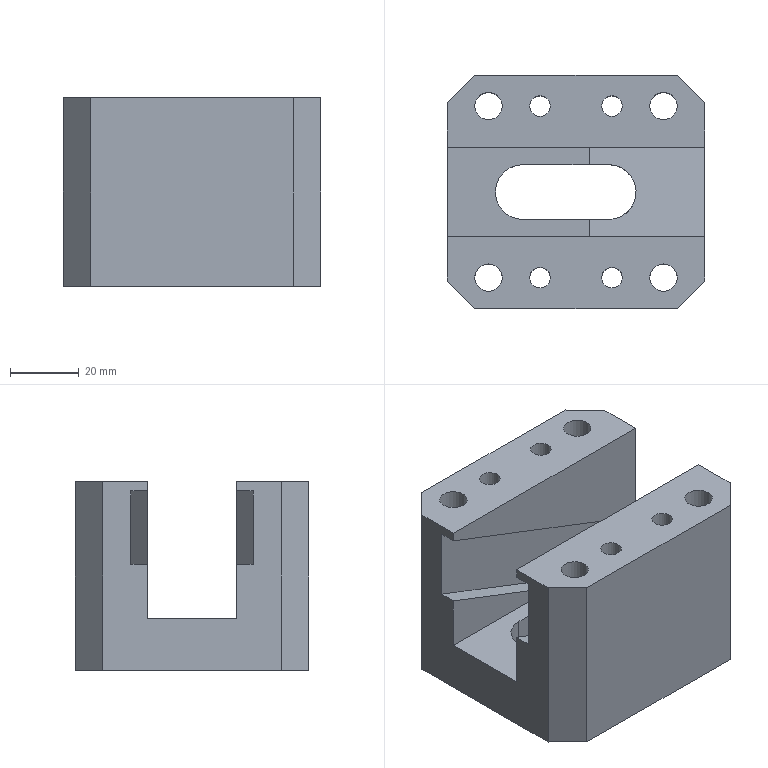Part | STEP file | P011002L001-003 | 1 solid | 41 faces | box 75 x 68 x 55 mm | volume 144794 mm3 | plane 27 | cylinder 14 | commonest cylinder face diameters 6 x4 8 x4 14 x4 16 x2